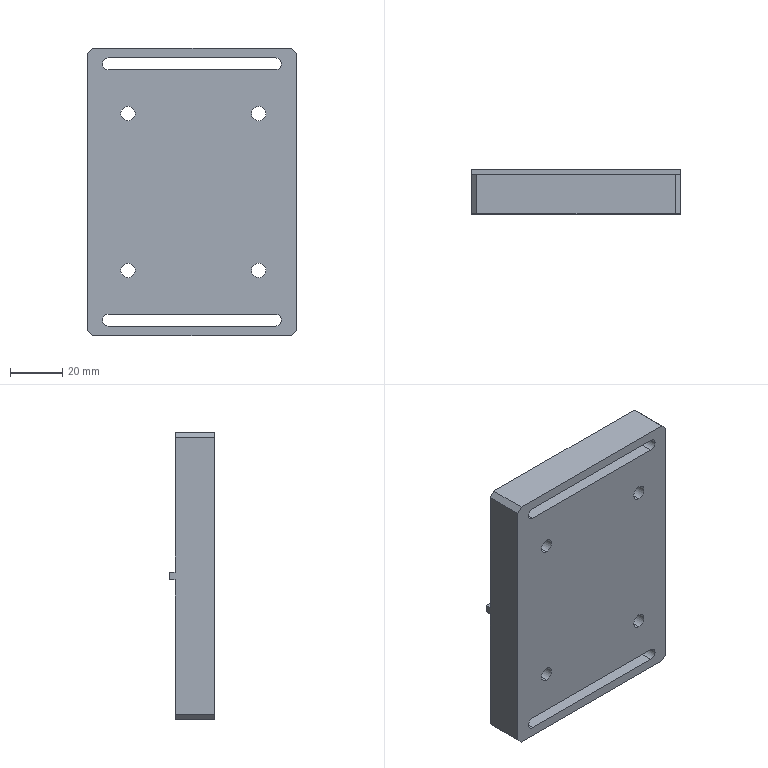Part | STEP file | 11-FG-S01111 | 1 solid | 44 faces | box 80 x 17 x 110 mm | volume 120634 mm3 | cylinder 22 | plane 22 | commonest cylinder face diameters 5.5 x8 10 x8 4.5 x6
STEP:
#1=CARTESIAN_POINT('',(-8.,15.,8.25));
#2=VERTEX_POINT('',#1);
#3=CARTESIAN_POINT('',(-5.75,15.,6.));
#4=VERTEX_POINT('',#3);
#5=CARTESIAN_POINT('',(-8.,15.,6.));
#6=DIRECTION('',(0.,1.,0.));
#7=DIRECTION('',(1.,0.,0.));
#8=AXIS2_PLACEMENT_3D('',#5,#6,#7);
#9=CIRCLE('',#8,2.25);
#10=EDGE_CURVE('',#2,#4,#9,.T.);
#11=ORIENTED_EDGE('',*,*,#10,.T.);
#12=CARTESIAN_POINT('',(-5.75,0.,6.));
#13=VERTEX_POINT('',#12);
#14=CARTESIAN_POINT('',(-5.75,444.,6.));
#15=DIRECTION('',(0.,-1.,0.));
#16=VECTOR('',#15,1000.);
#17=LINE('',#14,#16);
#18=EDGE_CURVE('',#4,#13,#17,.T.);
#19=ORIENTED_EDGE('',*,*,#18,.T.);
#20=CARTESIAN_POINT('',(-8.,0.,8.25));
#21=VERTEX_POINT('',#20);
#22=CARTESIAN_POINT('',(-8.,0.,6.));
#23=DIRECTION('',(0.,1.,0.));
#24=DIRECTION('',(1.,0.,0.));
#25=AXIS2_PLACEMENT_3D('',#22,#23,#24);
#26=CIRCLE('',#25,2.25);
#27=EDGE_CURVE('',#21,#13,#26,.T.);
#28=ORIENTED_EDGE('',*,*,#27,.F.);
#29=CARTESIAN_POINT('',(-8.,444.,8.25));
#30=DIRECTION('',(0.,-1.,0.));
#31=VECTOR('',#30,1000.);
#32=LINE('',#29,#31);
#33=EDGE_CURVE('',#2,#21,#32,.T.);
#34=ORIENTED_EDGE('',*,*,#33,.F.);
#35=EDGE_LOOP('',(#11,#19,#28,#34));
#36=FACE_OUTER_BOUND('',#35,.T.);
#37=CARTESIAN_POINT('',(-8.,444.,6.));
#38=DIRECTION('',(0.,-1.,0.));
#39=DIRECTION('',(1.,0.,0.));
#40=AXIS2_PLACEMENT_3D('',#37,#38,#39);
#41=CYLINDRICAL_SURFACE('',#40,2.25);
#42=ADVANCED_FACE('',(#36),#41,.F.);
#43=CARTESIAN_POINT('',(-5.75,15.,104.));
#44=VERTEX_POINT('',#43);
#45=CARTESIAN_POINT('',(-8.,15.,106.25));
#46=VERTEX_POINT('',#45);
#47=CARTESIAN_POINT('',(-8.,15.,104.));
#48=DIRECTION('',(0.,-1.,0.));
#49=DIRECTION('',(1.,0.,0.));
#50=AXIS2_PLACEMENT_3D('',#47,#48,#49);
#51=CIRCLE('',#50,2.25);
#52=EDGE_CURVE('',#44,#46,#51,.T.);
#53=ORIENTED_EDGE('',*,*,#52,.F.);
#54=CARTESIAN_POINT('',(-5.75,0.,104.));
#55=VERTEX_POINT('',#54);
#56=CARTESIAN_POINT('',(-5.75,444.,104.));
#57=DIRECTION('',(0.,-1.,0.));
#58=VECTOR('',#57,1000.);
#59=LINE('',#56,#58);
#60=EDGE_CURVE('',#44,#55,#59,.T.);
#61=ORIENTED_EDGE('',*,*,#60,.T.);
#62=CARTESIAN_POINT('',(-8.,0.,106.25));
#63=VERTEX_POINT('',#62);
#64=CARTESIAN_POINT('',(-8.,0.,104.));
#65=DIRECTION('',(0.,-1.,0.));
#66=DIRECTION('',(1.,0.,0.));
#67=AXIS2_PLACEMENT_3D('',#64,#65,#66);
#68=CIRCLE('',#67,2.25);
#69=EDGE_CURVE('',#55,#63,#68,.T.);
#70=ORIENTED_EDGE('',*,*,#69,.T.);
#71=CARTESIAN_POINT('',(-8.,444.,106.25));
#72=DIRECTION('',(0.,-1.,0.));
#73=VECTOR('',#72,1000.);
#74=LINE('',#71,#73);
#75=EDGE_CURVE('',#46,#63,#74,.T.);
#76=ORIENTED_EDGE('',*,*,#75,.F.);
#77=EDGE_LOOP('',(#53,#61,#70,#76));
#78=FACE_OUTER_BOUND('',#77,.T.);
#79=CARTESIAN_POINT('',(-8.,444.,104.));
#80=DIRECTION('',(0.,-1.,0.));
#81=DIRECTION('',(1.,0.,0.));
#82=AXIS2_PLACEMENT_3D('',#79,#80,#81);
#83=CYLINDRICAL_SURFACE('',#82,2.25);
#84=ADVANCED_FACE('',(#78),#83,.F.);
#85=CARTESIAN_POINT('',(-14.5,9.6,20.));
#86=VERTEX_POINT('',#85);
#87=CARTESIAN_POINT('',(-14.5,9.6,30.));
#88=VERTEX_POINT('',#87);
#89=CARTESIAN_POINT('',(-14.5,9.6,25.));
#90=DIRECTION('',(0.,1.,0.));
#91=DIRECTION('',(0.,0.,1.));
#92=AXIS2_PLACEMENT_3D('',#89,#90,#91);
#93=CIRCLE('',#92,5.);
#94=EDGE_CURVE('',#86,#88,#93,.T.);
#95=ORIENTED_EDGE('',*,*,#94,.F.);
#96=CARTESIAN_POINT('',(-14.5,15.,20.));
#97=VERTEX_POINT('',#96);
#98=CARTESIAN_POINT('',(-14.5,15.,20.));
#99=DIRECTION('',(0.,1.,0.));
#100=VECTOR('',#99,1000.);
#101=LINE('',#98,#100);
#102=EDGE_CURVE('',#86,#97,#101,.T.);
#103=ORIENTED_EDGE('',*,*,#102,.T.);
#104=CARTESIAN_POINT('',(-14.5,15.,30.));
#105=VERTEX_POINT('',#104);
#106=CARTESIAN_POINT('',(-14.5,15.,25.));
#107=DIRECTION('',(0.,1.,0.));
#108=DIRECTION('',(0.,0.,1.));
#109=AXIS2_PLACEMENT_3D('',#106,#107,#108);
#110=CIRCLE('',#109,5.);
#111=EDGE_CURVE('',#97,#105,#110,.T.);
#112=ORIENTED_EDGE('',*,*,#111,.T.);
#113=CARTESIAN_POINT('',(-14.5,15.,30.));
#114=DIRECTION('',(0.,1.,0.));
#115=VECTOR('',#114,1000.);
#116=LINE('',#113,#115);
#117=EDGE_CURVE('',#88,#105,#116,.T.);
#118=ORIENTED_EDGE('',*,*,#117,.F.);
#119=EDGE_LOOP('',(#95,#103,#112,#118));
#120=FACE_OUTER_BOUND('',#119,.T.);
#121=CARTESIAN_POINT('',(-14.5,15.,25.));
#122=DIRECTION('',(0.,1.,0.));
#123=DIRECTION('',(0.,0.,1.));
#124=AXIS2_PLACEMENT_3D('',#121,#122,#123);
#125=CYLINDRICAL_SURFACE('',#124,5.);
#126=ADVANCED_FACE('',(#120),#125,.F.);
#127=CARTESIAN_POINT('',(-14.5,0.,22.25));
#128=VERTEX_POINT('',#127);
#129=CARTESIAN_POINT('',(-14.5,0.,27.75));
#130=VERTEX_POINT('',#129);
#131=CARTESIAN_POINT('',(-14.5,0.,25.));
#132=DIRECTION('',(0.,1.,0.));
#133=DIRECTION('',(0.,0.,1.));
#134=AXIS2_PLACEMENT_3D('',#131,#132,#133);
#135=CIRCLE('',#134,2.75);
#136=EDGE_CURVE('',#128,#130,#135,.T.);
#137=ORIENTED_EDGE('',*,*,#136,.F.);
#138=CARTESIAN_POINT('',(-14.5,9.6,22.25));
#139=VERTEX_POINT('',#138);
#140=CARTESIAN_POINT('',(-14.5,15.,22.25));
#141=DIRECTION('',(0.,1.,0.));
#142=VECTOR('',#141,1000.);
#143=LINE('',#140,#142);
#144=EDGE_CURVE('',#128,#139,#143,.T.);
#145=ORIENTED_EDGE('',*,*,#144,.T.);
#146=CARTESIAN_POINT('',(-14.5,9.6,27.75));
#147=VERTEX_POINT('',#146);
#148=CARTESIAN_POINT('',(-14.5,9.6,25.));
#149=DIRECTION('',(0.,1.,0.));
#150=DIRECTION('',(0.,0.,1.));
#151=AXIS2_PLACEMENT_3D('',#148,#149,#150);
#152=CIRCLE('',#151,2.75);
#153=EDGE_CURVE('',#139,#147,#152,.T.);
#154=ORIENTED_EDGE('',*,*,#153,.T.);
#155=CARTESIAN_POINT('',(-14.5,15.,27.75));
#156=DIRECTION('',(0.,1.,0.));
#157=VECTOR('',#156,1000.);
#158=LINE('',#155,#157);
#159=EDGE_CURVE('',#130,#147,#158,.T.);
#160=ORIENTED_EDGE('',*,*,#159,.F.);
#161=EDGE_LOOP('',(#137,#145,#154,#160));
#162=FACE_OUTER_BOUND('',#161,.T.);
#163=CARTESIAN_POINT('',(-14.5,15.,25.));
#164=DIRECTION('',(0.,1.,0.));
#165=DIRECTION('',(0.,0.,1.));
#166=AXIS2_PLACEMENT_3D('',#163,#164,#165);
#167=CYLINDRICAL_SURFACE('',#166,2.75);
#168=ADVANCED_FACE('',(#162),#167,.F.);
#169=CARTESIAN_POINT('',(-14.5,9.6,80.));
#170=VERTEX_POINT('',#169);
#171=CARTESIAN_POINT('',(-14.5,9.6,90.));
#172=VERTEX_POINT('',#171);
#173=CARTESIAN_POINT('',(-14.5,9.6,85.));
#174=DIRECTION('',(0.,1.,0.));
#175=DIRECTION('',(0.,0.,1.));
#176=AXIS2_PLACEMENT_3D('',#173,#174,#175);
#177=CIRCLE('',#176,5.);
#178=EDGE_CURVE('',#170,#172,#177,.T.);
#179=ORIENTED_EDGE('',*,*,#178,.F.);
#180=CARTESIAN_POINT('',(-14.5,15.,80.));
#181=VERTEX_POINT('',#180);
#182=CARTESIAN_POINT('',(-14.5,15.,80.));
#183=DIRECTION('',(0.,1.,0.));
#184=VECTOR('',#183,1000.);
#185=LINE('',#182,#184);
#186=EDGE_CURVE('',#170,#181,#185,.T.);
#187=ORIENTED_EDGE('',*,*,#186,.T.);
#188=CARTESIAN_POINT('',(-14.5,15.,90.));
#189=VERTEX_POINT('',#188);
#190=CARTESIAN_POINT('',(-14.5,15.,85.));
#191=DIRECTION('',(0.,1.,0.));
#192=DIRECTION('',(0.,0.,1.));
#193=AXIS2_PLACEMENT_3D('',#190,#191,#192);
#194=CIRCLE('',#193,5.);
#195=EDGE_CURVE('',#181,#189,#194,.T.);
#196=ORIENTED_EDGE('',*,*,#195,.T.);
#197=CARTESIAN_POINT('',(-14.5,15.,90.));
#198=DIRECTION('',(0.,1.,0.));
#199=VECTOR('',#198,1000.);
#200=LINE('',#197,#199);
#201=EDGE_CURVE('',#172,#189,#200,.T.);
#202=ORIENTED_EDGE('',*,*,#201,.F.);
#203=EDGE_LOOP('',(#179,#187,#196,#202));
#204=FACE_OUTER_BOUND('',#203,.T.);
#205=CARTESIAN_POINT('',(-14.5,15.,85.));
#206=DIRECTION('',(0.,1.,0.));
#207=DIRECTION('',(0.,0.,1.));
#208=AXIS2_PLACEMENT_3D('',#205,#206,#207);
#209=CYLINDRICAL_SURFACE('',#208,5.);
#210=ADVANCED_FACE('',(#204),#209,.F.);
#211=CARTESIAN_POINT('',(-14.5,0.,82.25));
#212=VERTEX_POINT('',#211);
#213=CARTESIAN_POINT('',(-14.5,0.,87.75));
#214=VERTEX_POINT('',#213);
#215=CARTESIAN_POINT('',(-14.5,0.,85.));
#216=DIRECTION('',(0.,1.,0.));
#217=DIRECTION('',(0.,0.,1.));
#218=AXIS2_PLACEMENT_3D('',#215,#216,#217);
#219=CIRCLE('',#218,2.75);
#220=EDGE_CURVE('',#212,#214,#219,.T.);
#221=ORIENTED_EDGE('',*,*,#220,.F.);
#222=CARTESIAN_POINT('',(-14.5,9.6,82.25));
#223=VERTEX_POINT('',#222);
#224=CARTESIAN_POINT('',(-14.5,15.,82.25));
#225=DIRECTION('',(0.,1.,0.));
#226=VECTOR('',#225,1000.);
#227=LINE('',#224,#226);
#228=EDGE_CURVE('',#212,#223,#227,.T.);
#229=ORIENTED_EDGE('',*,*,#228,.T.);
#230=CARTESIAN_POINT('',(-14.5,9.6,87.75));
#231=VERTEX_POINT('',#230);
#232=CARTESIAN_POINT('',(-14.5,9.6,85.));
#233=DIRECTION('',(0.,1.,0.));
#234=DIRECTION('',(0.,0.,1.));
#235=AXIS2_PLACEMENT_3D('',#232,#233,#234);
#236=CIRCLE('',#235,2.75);
#237=EDGE_CURVE('',#223,#231,#236,.T.);
#238=ORIENTED_EDGE('',*,*,#237,.T.);
#239=CARTESIAN_POINT('',(-14.5,15.,87.75));
#240=DIRECTION('',(0.,1.,0.));
#241=VECTOR('',#240,1000.);
#242=LINE('',#239,#241);
#243=EDGE_CURVE('',#214,#231,#242,.T.);
#244=ORIENTED_EDGE('',*,*,#243,.F.);
#245=EDGE_LOOP('',(#221,#229,#238,#244));
#246=FACE_OUTER_BOUND('',#245,.T.);
#247=CARTESIAN_POINT('',(-14.5,15.,85.));
#248=DIRECTION('',(0.,1.,0.));
#249=DIRECTION('',(0.,0.,1.));
#250=AXIS2_PLACEMENT_3D('',#247,#248,#249);
#251=CYLINDRICAL_SURFACE('',#250,2.75);
#252=ADVANCED_FACE('',(#246),#251,.F.);
#253=CARTESIAN_POINT('',(-64.5,9.6,20.));
#254=VERTEX_POINT('',#253);
#255=CARTESIAN_POINT('',(-64.5,9.6,30.));
#256=VERTEX_POINT('',#255);
#257=CARTESIAN_POINT('',(-64.5,9.6,25.));
#258=DIRECTION('',(0.,1.,0.));
#259=DIRECTION('',(0.,0.,1.));
#260=AXIS2_PLACEMENT_3D('',#257,#258,#259);
#261=CIRCLE('',#260,5.);
#262=EDGE_CURVE('',#254,#256,#261,.T.);
#263=ORIENTED_EDGE('',*,*,#262,.F.);
#264=CARTESIAN_POINT('',(-64.5,15.,20.));
#265=VERTEX_POINT('',#264);
#266=CARTESIAN_POINT('',(-64.5,15.,20.));
#267=DIRECTION('',(0.,1.,0.));
#268=VECTOR('',#267,1000.);
#269=LINE('',#266,#268);
#270=EDGE_CURVE('',#254,#265,#269,.T.);
#271=ORIENTED_EDGE('',*,*,#270,.T.);
#272=CARTESIAN_POINT('',(-64.5,15.,30.));
#273=VERTEX_POINT('',#272);
#274=CARTESIAN_POINT('',(-64.5,15.,25.));
#275=DIRECTION('',(0.,1.,0.));
#276=DIRECTION('',(0.,0.,1.));
#277=AXIS2_PLACEMENT_3D('',#274,#275,#276);
#278=CIRCLE('',#277,5.);
#279=EDGE_CURVE('',#265,#273,#278,.T.);
#280=ORIENTED_EDGE('',*,*,#279,.T.);
#281=CARTESIAN_POINT('',(-64.5,15.,30.));
#282=DIRECTION('',(0.,1.,0.));
#283=VECTOR('',#282,1000.);
#284=LINE('',#281,#283);
#285=EDGE_CURVE('',#256,#273,#284,.T.);
#286=ORIENTED_EDGE('',*,*,#285,.F.);
#287=EDGE_LOOP('',(#263,#271,#280,#286));
#288=FACE_OUTER_BOUND('',#287,.T.);
#289=CARTESIAN_POINT('',(-64.5,15.,25.));
#290=DIRECTION('',(0.,1.,0.));
#291=DIRECTION('',(0.,0.,1.));
#292=AXIS2_PLACEMENT_3D('',#289,#290,#291);
#293=CYLINDRICAL_SURFACE('',#292,5.);
#294=ADVANCED_FACE('',(#288),#293,.F.);
#295=CARTESIAN_POINT('',(-64.5,0.,22.25));
#296=VERTEX_POINT('',#295);
#297=CARTESIAN_POINT('',(-64.5,0.,27.75));
#298=VERTEX_POINT('',#297);
#299=CARTESIAN_POINT('',(-64.5,0.,25.));
#300=DIRECTION('',(0.,1.,0.));
#301=DIRECTION('',(0.,0.,1.));
#302=AXIS2_PLACEMENT_3D('',#299,#300,#301);
#303=CIRCLE('',#302,2.75);
#304=EDGE_CURVE('',#296,#298,#303,.T.);
#305=ORIENTED_EDGE('',*,*,#304,.F.);
#306=CARTESIAN_POINT('',(-64.5,9.6,22.25));
#307=VERTEX_POINT('',#306);
#308=CARTESIAN_POINT('',(-64.5,15.,22.25));
#309=DIRECTION('',(0.,1.,0.));
#310=VECTOR('',#309,1000.);
#311=LINE('',#308,#310);
#312=EDGE_CURVE('',#296,#307,#311,.T.);
#313=ORIENTED_EDGE('',*,*,#312,.T.);
#314=CARTESIAN_POINT('',(-64.5,9.6,27.75));
#315=VERTEX_POINT('',#314);
#316=CARTESIAN_POINT('',(-64.5,9.6,25.));
#317=DIRECTION('',(0.,1.,0.));
#318=DIRECTION('',(0.,0.,1.));
#319=AXIS2_PLACEMENT_3D('',#316,#317,#318);
#320=CIRCLE('',#319,2.75);
#321=EDGE_CURVE('',#307,#315,#320,.T.);
#322=ORIENTED_EDGE('',*,*,#321,.T.);
#323=CARTESIAN_POINT('',(-64.5,15.,27.75));
#324=DIRECTION('',(0.,1.,0.));
#325=VECTOR('',#324,1000.);
#326=LINE('',#323,#325);
#327=EDGE_CURVE('',#298,#315,#326,.T.);
#328=ORIENTED_EDGE('',*,*,#327,.F.);
#329=EDGE_LOOP('',(#305,#313,#322,#328));
#330=FACE_OUTER_BOUND('',#329,.T.);
#331=CARTESIAN_POINT('',(-64.5,15.,25.));
#332=DIRECTION('',(0.,1.,0.));
#333=DIRECTION('',(0.,0.,1.));
#334=AXIS2_PLACEMENT_3D('',#331,#332,#333);
#335=CYLINDRICAL_SURFACE('',#334,2.75);
#336=ADVANCED_FACE('',(#330),#335,.F.);
#337=CARTESIAN_POINT('',(-64.5,9.6,80.));
#338=VERTEX_POINT('',#337);
#339=CARTESIAN_POINT('',(-64.5,9.6,90.));
#340=VERTEX_POINT('',#339);
#341=CARTESIAN_POINT('',(-64.5,9.6,85.));
#342=DIRECTION('',(0.,1.,0.));
#343=DIRECTION('',(0.,0.,1.));
#344=AXIS2_PLACEMENT_3D('',#341,#342,#343);
#345=CIRCLE('',#344,5.);
#346=EDGE_CURVE('',#338,#340,#345,.T.);
#347=ORIENTED_EDGE('',*,*,#346,.F.);
#348=CARTESIAN_POINT('',(-64.5,15.,80.));
#349=VERTEX_POINT('',#348);
#350=CARTESIAN_POINT('',(-64.5,15.,80.));
#351=DIRECTION('',(0.,1.,0.));
#352=VECTOR('',#351,1000.);
#353=LINE('',#350,#352);
#354=EDGE_CURVE('',#338,#349,#353,.T.);
#355=ORIENTED_EDGE('',*,*,#354,.T.);
#356=CARTESIAN_POINT('',(-64.5,15.,90.));
#357=VERTEX_POINT('',#356);
#358=CARTESIAN_POINT('',(-64.5,15.,85.));
#359=DIRECTION('',(0.,1.,0.));
#360=DIRECTION('',(0.,0.,1.));
#361=AXIS2_PLACEMENT_3D('',#358,#359,#360);
#362=CIRCLE('',#361,5.);
#363=EDGE_CURVE('',#349,#357,#362,.T.);
#364=ORIENTED_EDGE('',*,*,#363,.T.);
#365=CARTESIAN_POINT('',(-64.5,15.,90.));
#366=DIRECTION('',(0.,1.,0.));
#367=VECTOR('',#366,1000.);
#368=LINE('',#365,#367);
#369=EDGE_CURVE('',#340,#357,#368,.T.);
#370=ORIENTED_EDGE('',*,*,#369,.F.);
#371=EDGE_LOOP('',(#347,#355,#364,#370));
#372=FACE_OUTER_BOUND('',#371,.T.);
#373=CARTESIAN_POINT('',(-64.5,15.,85.));
#374=DIRECTION('',(0.,1.,0.));
#375=DIRECTION('',(0.,0.,1.));
#376=AXIS2_PLACEMENT_3D('',#373,#374,#375);
#377=CYLINDRICAL_SURFACE('',#376,5.);
#378=ADVANCED_FACE('',(#372),#377,.F.);
#379=CARTESIAN_POINT('',(-64.5,0.,82.25));
#380=VERTEX_POINT('',#379);
#381=CARTESIAN_POINT('',(-64.5,0.,87.75));
#382=VERTEX_POINT('',#381);
#383=CARTESIAN_POINT('',(-64.5,0.,85.));
#384=DIRECTION('',(0.,1.,0.));
#385=DIRECTION('',(0.,0.,1.));
#386=AXIS2_PLACEMENT_3D('',#383,#384,#385);
#387=CIRCLE('',#386,2.75);
#388=EDGE_CURVE('',#380,#382,#387,.T.);
#389=ORIENTED_EDGE('',*,*,#388,.F.);
#390=CARTESIAN_POINT('',(-64.5,9.6,82.25));
#391=VERTEX_POINT('',#390);
#392=CARTESIAN_POINT('',(-64.5,15.,82.25));
#393=DIRECTION('',(0.,1.,0.));
#394=VECTOR('',#393,1000.);
#395=LINE('',#392,#394);
#396=EDGE_CURVE('',#380,#391,#395,.T.);
#397=ORIENTED_EDGE('',*,*,#396,.T.);
#398=CARTESIAN_POINT('',(-64.5,9.6,87.75));
#399=VERTEX_POINT('',#398);
#400=CARTESIAN_POINT('',(-64.5,9.6,85.));
#401=DIRECTION('',(0.,1.,0.));
#402=DIRECTION('',(0.,0.,1.));
#403=AXIS2_PLACEMENT_3D('',#400,#401,#402);
#404=CIRCLE('',#403,2.75);
#405=EDGE_CURVE('',#391,#399,#404,.T.);
#406=ORIENTED_EDGE('',*,*,#405,.T.);
#407=CARTESIAN_POINT('',(-64.5,15.,87.75));
#408=DIRECTION('',(0.,1.,0.));
#409=VECTOR('',#408,1000.);
#410=LINE('',#407,#409);
#411=EDGE_CURVE('',#382,#399,#410,.T.);
#412=ORIENTED_EDGE('',*,*,#411,.F.);
#413=EDGE_LOOP('',(#389,#397,#406,#412));
#414=FACE_OUTER_BOUND('',#413,.T.);
#415=CARTESIAN_POINT('',(-64.5,15.,85.));
#416=DIRECTION('',(0.,1.,0.));
#417=DIRECTION('',(0.,0.,1.));
#418=AXIS2_PLACEMENT_3D('',#415,#416,#417);
#419=CYLINDRICAL_SURFACE('',#418,2.75);
#420=ADVANCED_FACE('',(#414),#419,.F.);
#421=CARTESIAN_POINT('',(-80.,15.,53.5));
#422=VERTEX_POINT('',#421);
#423=CARTESIAN_POINT('',(-80.,15.,2.));
#424=VERTEX_POINT('',#423);
#425=CARTESIAN_POINT('',(-80.,15.,110.));
#426=DIRECTION('',(0.,0.,-1.));
#427=VECTOR('',#426,1000.);
#428=LINE('',#425,#427);
#429=EDGE_CURVE('',#422,#424,#428,.T.);
#430=ORIENTED_EDGE('',*,*,#429,.F.);
#431=CARTESIAN_POINT('',(0.,15.,53.5));
#432=VERTEX_POINT('',#431);
#433=CARTESIAN_POINT('',(-83.606,15.,53.5));
#434=DIRECTION('',(1.,0.,0.));
#435=VECTOR('',#434,1000.);
#436=LINE('',#433,#435);
#437=EDGE_CURVE('',#422,#432,#436,.T.);
#438=ORIENTED_EDGE('',*,*,#437,.T.);
#439=CARTESIAN_POINT('',(0.,15.,2.));
#440=VERTEX_POINT('',#439);
#441=CARTESIAN_POINT('',(0.,15.,110.));
#442=DIRECTION('',(0.,0.,-1.));
#443=VECTOR('',#442,1000.);
#444=LINE('',#441,#443);
#445=EDGE_CURVE('',#432,#440,#444,.T.);
#446=ORIENTED_EDGE('',*,*,#445,.T.);
#447=CARTESIAN_POINT('',(-2.,15.,0.));
#448=VERTEX_POINT('',#447);
#449=CARTESIAN_POINT('',(0.,15.,2.));
#450=DIRECTION('',(-0.7071,0.,-0.7071));
#451=VECTOR('',#450,1000.);
#452=LINE('',#449,#451);
#453=EDGE_CURVE('',#440,#448,#452,.T.);
#454=ORIENTED_EDGE('',*,*,#453,.T.);
#455=CARTESIAN_POINT('',(-78.,15.,0.));
#456=VERTEX_POINT('',#455);
#457=CARTESIAN_POINT('',(0.,15.,0.));
#458=DIRECTION('',(-1.,0.,0.));
#459=VECTOR('',#458,1000.);
#460=LINE('',#457,#459);
#461=EDGE_CURVE('',#448,#456,#460,.T.);
#462=ORIENTED_EDGE('',*,*,#461,.T.);
#463=CARTESIAN_POINT('',(-80.,15.,2.));
#464=DIRECTION('',(-0.7071,0.,0.7071));
#465=VECTOR('',#464,1000.);
#466=LINE('',#463,#465);
#467=EDGE_CURVE('',#456,#424,#466,.T.);
#468=ORIENTED_EDGE('',*,*,#467,.T.);
#469=EDGE_LOOP('',(#430,#438,#446,#454,#462,#468));
#470=FACE_OUTER_BOUND('',#469,.T.);
#471=CARTESIAN_POINT('',(-64.5,15.,25.));
#472=DIRECTION('',(0.,1.,0.));
#473=DIRECTION('',(0.,0.,1.));
#474=AXIS2_PLACEMENT_3D('',#471,#472,#473);
#475=CIRCLE('',#474,5.);
#476=EDGE_CURVE('',#273,#265,#475,.T.);
#477=ORIENTED_EDGE('',*,*,#476,.F.);
#478=ORIENTED_EDGE('',*,*,#279,.F.);
#479=EDGE_LOOP('',(#477,#478));
#480=FACE_BOUND('',#479,.T.);
#481=CARTESIAN_POINT('',(-14.5,15.,25.));
#482=DIRECTION('',(0.,1.,0.));
#483=DIRECTION('',(0.,0.,1.));
#484=AXIS2_PLACEMENT_3D('',#481,#482,#483);
#485=CIRCLE('',#484,5.);
#486=EDGE_CURVE('',#105,#97,#485,.T.);
#487=ORIENTED_EDGE('',*,*,#486,.F.);
#488=ORIENTED_EDGE('',*,*,#111,.F.);
#489=EDGE_LOOP('',(#487,#488));
#490=FACE_BOUND('',#489,.T.);
#491=ORIENTED_EDGE('',*,*,#10,.F.);
#492=CARTESIAN_POINT('',(-72.,15.,8.25));
#493=VERTEX_POINT('',#492);
#494=CARTESIAN_POINT('',(0.,15.,8.25));
#495=DIRECTION('',(1.,0.,0.));
#496=VECTOR('',#495,1000.);
#497=LINE('',#494,#496);
#498=EDGE_CURVE('',#493,#2,#497,.T.);
#499=ORIENTED_EDGE('',*,*,#498,.F.);
#500=CARTESIAN_POINT('',(-72.,15.,3.75));
#501=VERTEX_POINT('',#500);
#502=CARTESIAN_POINT('',(-72.,15.,6.));
#503=DIRECTION('',(0.,1.,0.));
#504=DIRECTION('',(1.,0.,0.));
#505=AXIS2_PLACEMENT_3D('',#502,#503,#504);
#506=CIRCLE('',#505,2.25);
#507=EDGE_CURVE('',#501,#493,#506,.T.);
#508=ORIENTED_EDGE('',*,*,#507,.F.);
#509=CARTESIAN_POINT('',(-8.,15.,3.75));
#510=VERTEX_POINT('',#509);
#511=CARTESIAN_POINT('',(0.,15.,3.75));
#512=DIRECTION('',(-1.,0.,0.));
#513=VECTOR('',#512,1000.);
#514=LINE('',#511,#513);
#515=EDGE_CURVE('',#510,#501,#514,.T.);
#516=ORIENTED_EDGE('',*,*,#515,.F.);
#517=CARTESIAN_POINT('',(-8.,15.,6.));
#518=DIRECTION('',(0.,1.,0.));
#519=DIRECTION('',(1.,0.,0.));
#520=AXIS2_PLACEMENT_3D('',#517,#518,#519);
#521=CIRCLE('',#520,2.25);
#522=EDGE_CURVE('',#4,#510,#521,.T.);
#523=ORIENTED_EDGE('',*,*,#522,.F.);
#524=EDGE_LOOP('',(#491,#499,#508,#516,#523));
#525=FACE_BOUND('',#524,.T.);
#526=CARTESIAN_POINT('',(0.,15.,110.));
#527=DIRECTION('',(0.,-1.,0.));
#528=DIRECTION('',(1.,0.,0.));
#529=AXIS2_PLACEMENT_3D('',#526,#527,#528);
#530=PLANE('',#529);
#531=ADVANCED_FACE('',(#470,#480,#490,#525),#530,.F.);
#532=CARTESIAN_POINT('',(-78.,0.,110.));
#533=VERTEX_POINT('',#532);
#534=CARTESIAN_POINT('',(-2.,0.,110.));
#535=VERTEX_POINT('',#534);
#536=CARTESIAN_POINT('',(0.,0.,110.));
#537=DIRECTION('',(1.,0.,0.));
#538=VECTOR('',#537,1000.);
#539=LINE('',#536,#538);
#540=EDGE_CURVE('',#533,#535,#539,.T.);
#541=ORIENTED_EDGE('',*,*,#540,.F.);
#542=CARTESIAN_POINT('',(-80.,0.,108.));
#543=VERTEX_POINT('',#542);
#544=CARTESIAN_POINT('',(-78.,0.,110.));
#545=DIRECTION('',(-0.7071,0.,-0.7071));
#546=VECTOR('',#545,1000.);
#547=LINE('',#544,#546);
#548=EDGE_CURVE('',#533,#543,#547,.T.);
#549=ORIENTED_EDGE('',*,*,#548,.T.);
#550=CARTESIAN_POINT('',(-80.,0.,2.));
#551=VERTEX_POINT('',#550);
#552=CARTESIAN_POINT('',(-80.,0.,110.));
#553=DIRECTION('',(0.,0.,-1.));
#554=VECTOR('',#553,1000.);
#555=LINE('',#552,#554);
#556=EDGE_CURVE('',#543,#551,#555,.T.);
#557=ORIENTED_EDGE('',*,*,#556,.T.);
#558=CARTESIAN_POINT('',(-78.,0.,0.));
#559=VERTEX_POINT('',#558);
#560=CARTESIAN_POINT('',(-80.,0.,2.));
#561=DIRECTION('',(0.7071,0.,-0.7071));
#562=VECTOR('',#561,1000.);
#563=LINE('',#560,#562);
#564=EDGE_CURVE('',#551,#559,#563,.T.);
#565=ORIENTED_EDGE('',*,*,#564,.T.);
#566=CARTESIAN_POINT('',(-2.,0.,0.));
#567=VERTEX_POINT('',#566);
#568=CARTESIAN_POINT('',(0.,0.,0.));
#569=DIRECTION('',(1.,0.,0.));
#570=VECTOR('',#569,1000.);
#571=LINE('',#568,#570);
#572=EDGE_CURVE('',#559,#567,#571,.T.);
#573=ORIENTED_EDGE('',*,*,#572,.T.);
#574=CARTESIAN_POINT('',(0.,0.,2.));
#575=VERTEX_POINT('',#574);
#576=CARTESIAN_POINT('',(0.,0.,2.));
#577=DIRECTION('',(0.7071,0.,0.7071));
#578=VECTOR('',#577,1000.);
#579=LINE('',#576,#578);
#580=EDGE_CURVE('',#567,#575,#579,.T.);
#581=ORIENTED_EDGE('',*,*,#580,.T.);
#582=CARTESIAN_POINT('',(0.,0.,108.));
#583=VERTEX_POINT('',#582);
#584=CARTESIAN_POINT('',(0.,0.,110.));
#585=DIRECTION('',(0.,0.,-1.));
#586=VECTOR('',#585,1000.);
#587=LINE('',#584,#586);
#588=EDGE_CURVE('',#583,#575,#587,.T.);
#589=ORIENTED_EDGE('',*,*,#588,.F.);
#590=CARTESIAN_POINT('',(-2.,0.,110.));
#591=DIRECTION('',(-0.7071,0.,0.7071));
#592=VECTOR('',#591,1000.);
#593=LINE('',#590,#592);
#594=EDGE_CURVE('',#583,#535,#593,.T.);
#595=ORIENTED_EDGE('',*,*,#594,.T.);
#596=EDGE_LOOP('',(#541,#549,#557,#565,#573,#581,#589,#595));
#597=FACE_OUTER_BOUND('',#596,.T.);
#598=CARTESIAN_POINT('',(-64.5,0.,85.));
#599=DIRECTION('',(0.,1.,0.));
#600=DIRECTION('',(0.,0.,1.));
#601=AXIS2_PLACEMENT_3D('',#598,#599,#600);
#602=CIRCLE('',#601,2.75);
#603=EDGE_CURVE('',#382,#380,#602,.T.);
#604=ORIENTED_EDGE('',*,*,#603,.T.);
#605=ORIENTED_EDGE('',*,*,#388,.T.);
#606=EDGE_LOOP('',(#604,#605));
#607=FACE_BOUND('',#606,.T.);
#608=CARTESIAN_POINT('',(-64.5,0.,25.));
#609=DIRECTION('',(0.,1.,0.));
#610=DIRECTION('',(0.,0.,1.));
#611=AXIS2_PLACEMENT_3D('',#608,#609,#610);
#612=CIRCLE('',#611,2.75);
#613=EDGE_CURVE('',#298,#296,#612,.T.);
#614=ORIENTED_EDGE('',*,*,#613,.T.);
#615=ORIENTED_EDGE('',*,*,#304,.T.);
#616=EDGE_LOOP('',(#614,#615));
#617=FACE_BOUND('',#616,.T.);
#618=CARTESIAN_POINT('',(-14.5,0.,85.));
#619=DIRECTION('',(0.,1.,0.));
#620=DIRECTION('',(0.,0.,1.));
#621=AXIS2_PLACEMENT_3D('',#618,#619,#620);
#622=CIRCLE('',#621,2.75);
#623=EDGE_CURVE('',#214,#212,#622,.T.);
#624=ORIENTED_EDGE('',*,*,#623,.T.);
#625=ORIENTED_EDGE('',*,*,#220,.T.);
#626=EDGE_LOOP('',(#624,#625));
#627=FACE_BOUND('',#626,.T.);
#628=CARTESIAN_POINT('',(-14.5,0.,25.));
#629=DIRECTION('',(0.,1.,0.));
#630=DIRECTION('',(0.,0.,1.));
#631=AXIS2_PLACEMENT_3D('',#628,#629,#630);
#632=CIRCLE('',#631,2.75);
#633=EDGE_CURVE('',#130,#128,#632,.T.);
#634=ORIENTED_EDGE('',*,*,#633,.T.);
#635=ORIENTED_EDGE('',*,*,#136,.T.);
#636=EDGE_LOOP('',(#634,#635));
#637=FACE_BOUND('',#636,.T.);
#638=CARTESIAN_POINT('',(-72.,0.,106.25));
#639=VERTEX_POINT('',#638);
#640=CARTESIAN_POINT('',(-8.,0.,106.25));
#641=DIRECTION('',(-1.,0.,0.));
#642=VECTOR('',#641,1000.);
#643=LINE('',#640,#642);
#644=EDGE_CURVE('',#63,#639,#643,.T.);
#645=ORIENTED_EDGE('',*,*,#644,.F.);
#646=ORIENTED_EDGE('',*,*,#69,.F.);
#647=CARTESIAN_POINT('',(-8.,0.,101.75));
#648=VERTEX_POINT('',#647);
#649=CARTESIAN_POINT('',(-8.,0.,104.));
#650=DIRECTION('',(0.,-1.,0.));
#651=DIRECTION('',(1.,0.,0.));
#652=AXIS2_PLACEMENT_3D('',#649,#650,#651);
#653=CIRCLE('',#652,2.25);
#654=EDGE_CURVE('',#648,#55,#653,.T.);
#655=ORIENTED_EDGE('',*,*,#654,.F.);
#656=CARTESIAN_POINT('',(-72.,0.,101.75));
#657=VERTEX_POINT('',#656);
#658=CARTESIAN_POINT('',(-8.,0.,101.75));
#659=DIRECTION('',(1.,0.,0.));
#660=VECTOR('',#659,1000.);
#661=LINE('',#658,#660);
#662=EDGE_CURVE('',#657,#648,#661,.T.);
#663=ORIENTED_EDGE('',*,*,#662,.F.);
#664=CARTESIAN_POINT('',(-72.,0.,104.));
#665=DIRECTION('',(0.,-1.,0.));
#666=DIRECTION('',(1.,0.,0.));
#667=AXIS2_PLACEMENT_3D('',#664,#665,#666);
#668=CIRCLE('',#667,2.25);
#669=EDGE_CURVE('',#639,#657,#668,.T.);
#670=ORIENTED_EDGE('',*,*,#669,.F.);
#671=EDGE_LOOP('',(#645,#646,#655,#663,#670));
#672=FACE_BOUND('',#671,.T.);
#673=ORIENTED_EDGE('',*,*,#27,.T.);
#674=CARTESIAN_POINT('',(-8.,0.,3.75));
#675=VERTEX_POINT('',#674);
#676=CARTESIAN_POINT('',(-8.,0.,6.));
#677=DIRECTION('',(0.,1.,0.));
#678=DIRECTION('',(1.,0.,0.));
#679=AXIS2_PLACEMENT_3D('',#676,#677,#678);
#680=CIRCLE('',#679,2.25);
#681=EDGE_CURVE('',#13,#675,#680,.T.);
#682=ORIENTED_EDGE('',*,*,#681,.T.);
#683=CARTESIAN_POINT('',(-72.,0.,3.75));
#684=VERTEX_POINT('',#683);
#685=CARTESIAN_POINT('',(-8.,0.,3.75));
#686=DIRECTION('',(-1.,0.,0.));
#687=VECTOR('',#686,1000.);
#688=LINE('',#685,#687);
#689=EDGE_CURVE('',#675,#684,#688,.T.);
#690=ORIENTED_EDGE('',*,*,#689,.T.);
#691=CARTESIAN_POINT('',(-72.,0.,8.25));
#692=VERTEX_POINT('',#691);
#693=CARTESIAN_POINT('',(-72.,0.,6.));
#694=DIRECTION('',(0.,1.,0.));
#695=DIRECTION('',(1.,0.,0.));
#696=AXIS2_PLACEMENT_3D('',#693,#694,#695);
#697=CIRCLE('',#696,2.25);
#698=EDGE_CURVE('',#684,#692,#697,.T.);
#699=ORIENTED_EDGE('',*,*,#698,.T.);
#700=CARTESIAN_POINT('',(-8.,0.,8.25));
#701=DIRECTION('',(1.,0.,0.));
#702=VECTOR('',#701,1000.);
#703=LINE('',#700,#702);
#704=EDGE_CURVE('',#692,#21,#703,.T.);
#705=ORIENTED_EDGE('',*,*,#704,.T.);
#706=EDGE_LOOP('',(#673,#682,#690,#699,#705));
#707=FACE_BOUND('',#706,.T.);
#708=CARTESIAN_POINT('',(0.,0.,110.));
#709=DIRECTION('',(0.,1.,0.));
#710=DIRECTION('',(-1.,0.,0.));
#711=AXIS2_PLACEMENT_3D('',#708,#709,#710);
#712=PLANE('',#711);
#713=ADVANCED_FACE('',(#597,#607,#617,#627,#637,#672,#707),#712,.F.);
#714=CARTESIAN_POINT('',(-72.,15.,101.75));
#715=VERTEX_POINT('',#714);
#716=CARTESIAN_POINT('',(-8.,15.,101.75));
#717=VERTEX_POINT('',#716);
#718=CARTESIAN_POINT('',(0.,15.,101.75));
#719=DIRECTION('',(1.,0.,0.));
#720=VECTOR('',#719,1000.);
#721=LINE('',#718,#720);
#722=EDGE_CURVE('',#715,#717,#721,.T.);
#723=ORIENTED_EDGE('',*,*,#722,.T.);
#724=CARTESIAN_POINT('',(-8.,15.,104.));
#725=DIRECTION('',(0.,-1.,0.));
#726=DIRECTION('',(1.,0.,0.));
#727=AXIS2_PLACEMENT_3D('',#724,#725,#726);
#728=CIRCLE('',#727,2.25);
#729=EDGE_CURVE('',#717,#44,#728,.T.);
#730=ORIENTED_EDGE('',*,*,#729,.T.);
#731=ORIENTED_EDGE('',*,*,#52,.T.);
#732=CARTESIAN_POINT('',(-72.,15.,106.25));
#733=VERTEX_POINT('',#732);
#734=CARTESIAN_POINT('',(0.,15.,106.25));
#735=DIRECTION('',(-1.,0.,0.));
#736=VECTOR('',#735,1000.);
#737=LINE('',#734,#736);
#738=EDGE_CURVE('',#46,#733,#737,.T.);
#739=ORIENTED_EDGE('',*,*,#738,.T.);
#740=CARTESIAN_POINT('',(-72.,15.,104.));
#741=DIRECTION('',(0.,-1.,0.));
#742=DIRECTION('',(1.,0.,0.));
#743=AXIS2_PLACEMENT_3D('',#740,#741,#742);
#744=CIRCLE('',#743,2.25);
#745=EDGE_CURVE('',#733,#715,#744,.T.);
#746=ORIENTED_EDGE('',*,*,#745,.T.);
#747=EDGE_LOOP('',(#723,#730,#731,#739,#746));
#748=FACE_BOUND('',#747,.T.);
#749=CARTESIAN_POINT('',(-64.5,15.,85.));
#750=DIRECTION('',(0.,1.,0.));
#751=DIRECTION('',(0.,0.,1.));
#752=AXIS2_PLACEMENT_3D('',#749,#750,#751);
#753=CIRCLE('',#752,5.);
#754=EDGE_CURVE('',#357,#349,#753,.T.);
#755=ORIENTED_EDGE('',*,*,#754,.F.);
#756=ORIENTED_EDGE('',*,*,#363,.F.);
#757=EDGE_LOOP('',(#755,#756));
#758=FACE_BOUND('',#757,.T.);
#759=CARTESIAN_POINT('',(-14.5,15.,85.));
#760=DIRECTION('',(0.,1.,0.));
#761=DIRECTION('',(0.,0.,1.));
#762=AXIS2_PLACEMENT_3D('',#759,#760,#761);
#763=CIRCLE('',#762,5.);
#764=EDGE_CURVE('',#189,#181,#763,.T.);
#765=ORIENTED_EDGE('',*,*,#764,.F.);
#766=ORIENTED_EDGE('',*,*,#195,.F.);
#767=EDGE_LOOP('',(#765,#766));
#768=FACE_BOUND('',#767,.T.);
#769=CARTESIAN_POINT('',(-80.,15.,56.5));
#770=VERTEX_POINT('',#769);
#771=CARTESIAN_POINT('',(0.,15.,56.5));
#772=VERTEX_POINT('',#771);
#773=CARTESIAN_POINT('',(-83.606,15.,56.5));
#774=DIRECTION('',(1.,0.,0.));
#775=VECTOR('',#774,1000.);
#776=LINE('',#773,#775);
#777=EDGE_CURVE('',#770,#772,#776,.T.);
#778=ORIENTED_EDGE('',*,*,#777,.F.);
#779=CARTESIAN_POINT('',(-80.,15.,108.));
#780=VERTEX_POINT('',#779);
#781=CARTESIAN_POINT('',(-80.,15.,110.));
#782=DIRECTION('',(0.,0.,-1.));
#783=VECTOR('',#782,1000.);
#784=LINE('',#781,#783);
#785=EDGE_CURVE('',#780,#770,#784,.T.);
#786=ORIENTED_EDGE('',*,*,#785,.F.);
#787=CARTESIAN_POINT('',(-78.,15.,110.));
#788=VERTEX_POINT('',#787);
#789=CARTESIAN_POINT('',(-78.,15.,110.));
#790=DIRECTION('',(0.7071,0.,0.7071));
#791=VECTOR('',#790,1000.);
#792=LINE('',#789,#791);
#793=EDGE_CURVE('',#780,#788,#792,.T.);
#794=ORIENTED_EDGE('',*,*,#793,.T.);
#795=CARTESIAN_POINT('',(-2.,15.,110.));
#796=VERTEX_POINT('',#795);
#797=CARTESIAN_POINT('',(0.,15.,110.));
#798=DIRECTION('',(-1.,0.,0.));
#799=VECTOR('',#798,1000.);
#800=LINE('',#797,#799);
#801=EDGE_CURVE('',#796,#788,#800,.T.);
#802=ORIENTED_EDGE('',*,*,#801,.F.);
#803=CARTESIAN_POINT('',(0.,15.,108.));
#804=VERTEX_POINT('',#803);
#805=CARTESIAN_POINT('',(-2.,15.,110.));
#806=DIRECTION('',(0.7071,0.,-0.7071));
#807=VECTOR('',#806,1000.);
#808=LINE('',#805,#807);
#809=EDGE_CURVE('',#796,#804,#808,.T.);
#810=ORIENTED_EDGE('',*,*,#809,.T.);
#811=CARTESIAN_POINT('',(0.,15.,110.));
#812=DIRECTION('',(0.,0.,-1.));
#813=VECTOR('',#812,1000.);
#814=LINE('',#811,#813);
#815=EDGE_CURVE('',#804,#772,#814,.T.);
#816=ORIENTED_EDGE('',*,*,#815,.T.);
#817=EDGE_LOOP('',(#778,#786,#794,#802,#810,#816));
#818=FACE_OUTER_BOUND('',#817,.T.);
#819=CARTESIAN_POINT('',(0.,15.,110.));
#820=DIRECTION('',(0.,-1.,0.));
#821=DIRECTION('',(1.,0.,0.));
#822=AXIS2_PLACEMENT_3D('',#819,#820,#821);
#823=PLANE('',#822);
#824=ADVANCED_FACE('',(#748,#758,#768,#818),#823,.F.);
#825=ORIENTED_EDGE('',*,*,#815,.F.);
#826=CARTESIAN_POINT('',(0.,0.,108.));
#827=DIRECTION('',(0.,-1.,0.));
#828=VECTOR('',#827,1000.);
#829=LINE('',#826,#828);
#830=EDGE_CURVE('',#804,#583,#829,.T.);
#831=ORIENTED_EDGE('',*,*,#830,.T.);
#832=ORIENTED_EDGE('',*,*,#588,.T.);
#833=CARTESIAN_POINT('',(0.,0.,2.));
#834=DIRECTION('',(0.,1.,0.));
#835=VECTOR('',#834,1000.);
#836=LINE('',#833,#835);
#837=EDGE_CURVE('',#575,#440,#836,.T.);
#838=ORIENTED_EDGE('',*,*,#837,.T.);
#839=ORIENTED_EDGE('',*,*,#445,.F.);
#840=CARTESIAN_POINT('',(0.,17.,53.5));
#841=VERTEX_POINT('',#840);
#842=CARTESIAN_POINT('',(0.,15.,53.5));
#843=DIRECTION('',(0.,1.,0.));
#844=VECTOR('',#843,1000.);
#845=LINE('',#842,#844);
#846=EDGE_CURVE('',#432,#841,#845,.T.);
#847=ORIENTED_EDGE('',*,*,#846,.T.);
#848=CARTESIAN_POINT('',(0.,17.,56.5));
#849=VERTEX_POINT('',#848);
#850=CARTESIAN_POINT('',(0.,17.,53.5));
#851=DIRECTION('',(0.,0.,1.));
#852=VECTOR('',#851,1000.);
#853=LINE('',#850,#852);
#854=EDGE_CURVE('',#841,#849,#853,.T.);
#855=ORIENTED_EDGE('',*,*,#854,.T.);
#856=CARTESIAN_POINT('',(0.,15.,56.5));
#857=DIRECTION('',(0.,-1.,0.));
#858=VECTOR('',#857,1000.);
#859=LINE('',#856,#858);
#860=EDGE_CURVE('',#849,#772,#859,.T.);
#861=ORIENTED_EDGE('',*,*,#860,.T.);
#862=EDGE_LOOP('',(#825,#831,#832,#838,#839,#847,#855,#861));
#863=FACE_OUTER_BOUND('',#862,.T.);
#864=CARTESIAN_POINT('',(0.,0.,110.));
#865=DIRECTION('',(-1.,0.,0.));
#866=DIRECTION('',(0.,0.,1.));
#867=AXIS2_PLACEMENT_3D('',#864,#865,#866);
#868=PLANE('',#867);
#869=ADVANCED_FACE('',(#863),#868,.F.);
#870=ORIENTED_EDGE('',*,*,#556,.F.);
#871=CARTESIAN_POINT('',(-80.,15.,108.));
#872=DIRECTION('',(0.,1.,0.));
#873=VECTOR('',#872,1000.);
#874=LINE('',#871,#873);
#875=EDGE_CURVE('',#543,#780,#874,.T.);
#876=ORIENTED_EDGE('',*,*,#875,.T.);
#877=ORIENTED_EDGE('',*,*,#785,.T.);
#878=CARTESIAN_POINT('',(-80.,17.,56.5));
#879=VERTEX_POINT('',#878);
#880=CARTESIAN_POINT('',(-80.,15.,56.5));
#881=DIRECTION('',(0.,1.,0.));
#882=VECTOR('',#881,1000.);
#883=LINE('',#880,#882);
#884=EDGE_CURVE('',#770,#879,#883,.T.);
#885=ORIENTED_EDGE('',*,*,#884,.T.);
#886=CARTESIAN_POINT('',(-80.,17.,53.5));
#887=VERTEX_POINT('',#886);
#888=CARTESIAN_POINT('',(-80.,17.,53.5));
#889=DIRECTION('',(0.,0.,-1.));
#890=VECTOR('',#889,1000.);
#891=LINE('',#888,#890);
#892=EDGE_CURVE('',#879,#887,#891,.T.);
#893=ORIENTED_EDGE('',*,*,#892,.T.);
#894=CARTESIAN_POINT('',(-80.,15.,53.5));
#895=DIRECTION('',(0.,-1.,0.));
#896=VECTOR('',#895,1000.);
#897=LINE('',#894,#896);
#898=EDGE_CURVE('',#887,#422,#897,.T.);
#899=ORIENTED_EDGE('',*,*,#898,.T.);
#900=ORIENTED_EDGE('',*,*,#429,.T.);
#901=CARTESIAN_POINT('',(-80.,0.,2.));
#902=DIRECTION('',(0.,-1.,0.));
#903=VECTOR('',#902,1000.);
#904=LINE('',#901,#903);
#905=EDGE_CURVE('',#424,#551,#904,.T.);
#906=ORIENTED_EDGE('',*,*,#905,.T.);
#907=EDGE_LOOP('',(#870,#876,#877,#885,#893,#899,#900,#906));
#908=FACE_OUTER_BOUND('',#907,.T.);
#909=CARTESIAN_POINT('',(-80.,0.,110.));
#910=DIRECTION('',(1.,0.,0.));
#911=DIRECTION('',(0.,0.,-1.));
#912=AXIS2_PLACEMENT_3D('',#909,#910,#911);
#913=PLANE('',#912);
#914=ADVANCED_FACE('',(#908),#913,.F.);
#915=ORIENTED_EDGE('',*,*,#801,.T.);
#916=CARTESIAN_POINT('',(-78.,0.,110.));
#917=DIRECTION('',(0.,-1.,0.));
#918=VECTOR('',#917,1000.);
#919=LINE('',#916,#918);
#920=EDGE_CURVE('',#788,#533,#919,.T.);
#921=ORIENTED_EDGE('',*,*,#920,.T.);
#922=ORIENTED_EDGE('',*,*,#540,.T.);
#923=CARTESIAN_POINT('',(-2.,15.,110.));
#924=DIRECTION('',(0.,1.,0.));
#925=VECTOR('',#924,1000.);
#926=LINE('',#923,#925);
#927=EDGE_CURVE('',#535,#796,#926,.T.);
#928=ORIENTED_EDGE('',*,*,#927,.T.);
#929=EDGE_LOOP('',(#915,#921,#922,#928));
#930=FACE_OUTER_BOUND('',#929,.T.);
#931=CARTESIAN_POINT('',(0.,15.,110.));
#932=DIRECTION('',(0.,0.,1.));
#933=DIRECTION('',(1.,0.,0.));
#934=AXIS2_PLACEMENT_3D('',#931,#932,#933);
#935=PLANE('',#934);
#936=ADVANCED_FACE('',(#930),#935,.T.);
#937=ORIENTED_EDGE('',*,*,#572,.F.);
#938=CARTESIAN_POINT('',(-78.,15.,0.));
#939=DIRECTION('',(0.,1.,0.));
#940=VECTOR('',#939,1000.);
#941=LINE('',#938,#940);
#942=EDGE_CURVE('',#559,#456,#941,.T.);
#943=ORIENTED_EDGE('',*,*,#942,.T.);
#944=ORIENTED_EDGE('',*,*,#461,.F.);
#945=CARTESIAN_POINT('',(-2.,15.,0.));
#946=DIRECTION('',(0.,-1.,0.));
#947=VECTOR('',#946,1000.);
#948=LINE('',#945,#947);
#949=EDGE_CURVE('',#448,#567,#948,.T.);
#950=ORIENTED_EDGE('',*,*,#949,.T.);
#951=EDGE_LOOP('',(#937,#943,#944,#950));
#952=FACE_OUTER_BOUND('',#951,.T.);
#953=CARTESIAN_POINT('',(0.,15.,0.));
#954=DIRECTION('',(0.,0.,1.));
#955=DIRECTION('',(1.,0.,0.));
#956=AXIS2_PLACEMENT_3D('',#953,#954,#955);
#957=PLANE('',#956);
#958=ADVANCED_FACE('',(#952),#957,.F.);
#959=ORIENTED_EDGE('',*,*,#793,.F.);
#960=ORIENTED_EDGE('',*,*,#875,.F.);
#961=ORIENTED_EDGE('',*,*,#548,.F.);
#962=ORIENTED_EDGE('',*,*,#920,.F.);
#963=EDGE_LOOP('',(#959,#960,#961,#962));
#964=FACE_OUTER_BOUND('',#963,.T.);
#965=CARTESIAN_POINT('',(-78.,15.,110.));
#966=DIRECTION('',(-0.7071,0.,0.7071));
#967=DIRECTION('',(0.,1.,0.));
#968=AXIS2_PLACEMENT_3D('',#965,#966,#967);
#969=PLANE('',#968);
#970=ADVANCED_FACE('',(#964),#969,.T.);
#971=ORIENTED_EDGE('',*,*,#467,.F.);
#972=ORIENTED_EDGE('',*,*,#942,.F.);
#973=ORIENTED_EDGE('',*,*,#564,.F.);
#974=ORIENTED_EDGE('',*,*,#905,.F.);
#975=EDGE_LOOP('',(#971,#972,#973,#974));
#976=FACE_OUTER_BOUND('',#975,.T.);
#977=CARTESIAN_POINT('',(-80.,0.,2.));
#978=DIRECTION('',(0.7071,0.,0.7071));
#979=DIRECTION('',(0.,-1.,0.));
#980=AXIS2_PLACEMENT_3D('',#977,#978,#979);
#981=PLANE('',#980);
#982=ADVANCED_FACE('',(#976),#981,.F.);
#983=ORIENTED_EDGE('',*,*,#594,.F.);
#984=ORIENTED_EDGE('',*,*,#830,.F.);
#985=ORIENTED_EDGE('',*,*,#809,.F.);
#986=ORIENTED_EDGE('',*,*,#927,.F.);
#987=EDGE_LOOP('',(#983,#984,#985,#986));
#988=FACE_OUTER_BOUND('',#987,.T.);
#989=CARTESIAN_POINT('',(-2.,15.,110.));
#990=DIRECTION('',(0.7071,0.,0.7071));
#991=DIRECTION('',(0.,-1.,0.));
#992=AXIS2_PLACEMENT_3D('',#989,#990,#991);
#993=PLANE('',#992);
#994=ADVANCED_FACE('',(#988),#993,.T.);
#995=ORIENTED_EDGE('',*,*,#580,.F.);
#996=ORIENTED_EDGE('',*,*,#949,.F.);
#997=ORIENTED_EDGE('',*,*,#453,.F.);
#998=ORIENTED_EDGE('',*,*,#837,.F.);
#999=EDGE_LOOP('',(#995,#996,#997,#998));
#1000=FACE_OUTER_BOUND('',#999,.T.);
#1001=CARTESIAN_POINT('',(0.,0.,2.));
#1002=DIRECTION('',(-0.7071,0.,0.7071));
#1003=DIRECTION('',(0.,1.,0.));
#1004=AXIS2_PLACEMENT_3D('',#1001,#1002,#1003);
#1005=PLANE('',#1004);
#1006=ADVANCED_FACE('',(#1000),#1005,.F.);
#1007=ORIENTED_EDGE('',*,*,#396,.F.);
#1008=ORIENTED_EDGE('',*,*,#603,.F.);
#1009=ORIENTED_EDGE('',*,*,#411,.T.);
#1010=CARTESIAN_POINT('',(-64.5,9.6,85.));
#1011=DIRECTION('',(0.,1.,0.));
#1012=DIRECTION('',(0.,0.,1.));
#1013=AXIS2_PLACEMENT_3D('',#1010,#1011,#1012);
#1014=CIRCLE('',#1013,2.75);
#1015=EDGE_CURVE('',#399,#391,#1014,.T.);
#1016=ORIENTED_EDGE('',*,*,#1015,.T.);
#1017=EDGE_LOOP('',(#1007,#1008,#1009,#1016));
#1018=FACE_OUTER_BOUND('',#1017,.T.);
#1019=CARTESIAN_POINT('',(-64.5,15.,85.));
#1020=DIRECTION('',(0.,1.,0.));
#1021=DIRECTION('',(0.,0.,1.));
#1022=AXIS2_PLACEMENT_3D('',#1019,#1020,#1021);
#1023=CYLINDRICAL_SURFACE('',#1022,2.75);
#1024=ADVANCED_FACE('',(#1018),#1023,.F.);
#1025=ORIENTED_EDGE('',*,*,#1015,.F.);
#1026=ORIENTED_EDGE('',*,*,#405,.F.);
#1027=EDGE_LOOP('',(#1025,#1026));
#1028=FACE_BOUND('',#1027,.T.);
#1029=CARTESIAN_POINT('',(-64.5,9.6,85.));
#1030=DIRECTION('',(0.,1.,0.));
#1031=DIRECTION('',(0.,0.,1.));
#1032=AXIS2_PLACEMENT_3D('',#1029,#1030,#1031);
#1033=CIRCLE('',#1032,5.);
#1034=EDGE_CURVE('',#340,#338,#1033,.T.);
#1035=ORIENTED_EDGE('',*,*,#1034,.T.);
#1036=ORIENTED_EDGE('',*,*,#346,.T.);
#1037=EDGE_LOOP('',(#1035,#1036));
#1038=FACE_OUTER_BOUND('',#1037,.T.);
#1039=CARTESIAN_POINT('',(-61.75,9.6,85.));
#1040=DIRECTION('',(0.,-1.,0.));
#1041=DIRECTION('',(0.,0.,-1.));
#1042=AXIS2_PLACEMENT_3D('',#1039,#1040,#1041);
#1043=PLANE('',#1042);
#1044=ADVANCED_FACE('',(#1028,#1038),#1043,.F.);
#1045=ORIENTED_EDGE('',*,*,#354,.F.);
#1046=ORIENTED_EDGE('',*,*,#1034,.F.);
#1047=ORIENTED_EDGE('',*,*,#369,.T.);
#1048=ORIENTED_EDGE('',*,*,#754,.T.);
#1049=EDGE_LOOP('',(#1045,#1046,#1047,#1048));
#1050=FACE_OUTER_BOUND('',#1049,.T.);
#1051=CARTESIAN_POINT('',(-64.5,15.,85.));
#1052=DIRECTION('',(0.,1.,0.));
#1053=DIRECTION('',(0.,0.,1.));
#1054=AXIS2_PLACEMENT_3D('',#1051,#1052,#1053);
#1055=CYLINDRICAL_SURFACE('',#1054,5.);
#1056=ADVANCED_FACE('',(#1050),#1055,.F.);
#1057=ORIENTED_EDGE('',*,*,#312,.F.);
#1058=ORIENTED_EDGE('',*,*,#613,.F.);
#1059=ORIENTED_EDGE('',*,*,#327,.T.);
#1060=CARTESIAN_POINT('',(-64.5,9.6,25.));
#1061=DIRECTION('',(0.,1.,0.));
#1062=DIRECTION('',(0.,0.,1.));
#1063=AXIS2_PLACEMENT_3D('',#1060,#1061,#1062);
#1064=CIRCLE('',#1063,2.75);
#1065=EDGE_CURVE('',#315,#307,#1064,.T.);
#1066=ORIENTED_EDGE('',*,*,#1065,.T.);
#1067=EDGE_LOOP('',(#1057,#1058,#1059,#1066));
#1068=FACE_OUTER_BOUND('',#1067,.T.);
#1069=CARTESIAN_POINT('',(-64.5,15.,25.));
#1070=DIRECTION('',(0.,1.,0.));
#1071=DIRECTION('',(0.,0.,1.));
#1072=AXIS2_PLACEMENT_3D('',#1069,#1070,#1071);
#1073=CYLINDRICAL_SURFACE('',#1072,2.75);
#1074=ADVANCED_FACE('',(#1068),#1073,.F.);
#1075=ORIENTED_EDGE('',*,*,#1065,.F.);
#1076=ORIENTED_EDGE('',*,*,#321,.F.);
#1077=EDGE_LOOP('',(#1075,#1076));
#1078=FACE_BOUND('',#1077,.T.);
#1079=CARTESIAN_POINT('',(-64.5,9.6,25.));
#1080=DIRECTION('',(0.,1.,0.));
#1081=DIRECTION('',(0.,0.,1.));
#1082=AXIS2_PLACEMENT_3D('',#1079,#1080,#1081);
#1083=CIRCLE('',#1082,5.);
#1084=EDGE_CURVE('',#256,#254,#1083,.T.);
#1085=ORIENTED_EDGE('',*,*,#1084,.T.);
#1086=ORIENTED_EDGE('',*,*,#262,.T.);
#1087=EDGE_LOOP('',(#1085,#1086));
#1088=FACE_OUTER_BOUND('',#1087,.T.);
#1089=CARTESIAN_POINT('',(-61.75,9.6,25.));
#1090=DIRECTION('',(0.,-1.,0.));
#1091=DIRECTION('',(0.,0.,-1.));
#1092=AXIS2_PLACEMENT_3D('',#1089,#1090,#1091);
#1093=PLANE('',#1092);
#1094=ADVANCED_FACE('',(#1078,#1088),#1093,.F.);
#1095=ORIENTED_EDGE('',*,*,#270,.F.);
#1096=ORIENTED_EDGE('',*,*,#1084,.F.);
#1097=ORIENTED_EDGE('',*,*,#285,.T.);
#1098=ORIENTED_EDGE('',*,*,#476,.T.);
#1099=EDGE_LOOP('',(#1095,#1096,#1097,#1098));
#1100=FACE_OUTER_BOUND('',#1099,.T.);
#1101=CARTESIAN_POINT('',(-64.5,15.,25.));
#1102=DIRECTION('',(0.,1.,0.));
#1103=DIRECTION('',(0.,0.,1.));
#1104=AXIS2_PLACEMENT_3D('',#1101,#1102,#1103);
#1105=CYLINDRICAL_SURFACE('',#1104,5.);
#1106=ADVANCED_FACE('',(#1100),#1105,.F.);
#1107=ORIENTED_EDGE('',*,*,#228,.F.);
#1108=ORIENTED_EDGE('',*,*,#623,.F.);
#1109=ORIENTED_EDGE('',*,*,#243,.T.);
#1110=CARTESIAN_POINT('',(-14.5,9.6,85.));
#1111=DIRECTION('',(0.,1.,0.));
#1112=DIRECTION('',(0.,0.,1.));
#1113=AXIS2_PLACEMENT_3D('',#1110,#1111,#1112);
#1114=CIRCLE('',#1113,2.75);
#1115=EDGE_CURVE('',#231,#223,#1114,.T.);
#1116=ORIENTED_EDGE('',*,*,#1115,.T.);
#1117=EDGE_LOOP('',(#1107,#1108,#1109,#1116));
#1118=FACE_OUTER_BOUND('',#1117,.T.);
#1119=CARTESIAN_POINT('',(-14.5,15.,85.));
#1120=DIRECTION('',(0.,1.,0.));
#1121=DIRECTION('',(0.,0.,1.));
#1122=AXIS2_PLACEMENT_3D('',#1119,#1120,#1121);
#1123=CYLINDRICAL_SURFACE('',#1122,2.75);
#1124=ADVANCED_FACE('',(#1118),#1123,.F.);
#1125=ORIENTED_EDGE('',*,*,#1115,.F.);
#1126=ORIENTED_EDGE('',*,*,#237,.F.);
#1127=EDGE_LOOP('',(#1125,#1126));
#1128=FACE_BOUND('',#1127,.T.);
#1129=CARTESIAN_POINT('',(-14.5,9.6,85.));
#1130=DIRECTION('',(0.,1.,0.));
#1131=DIRECTION('',(0.,0.,1.));
#1132=AXIS2_PLACEMENT_3D('',#1129,#1130,#1131);
#1133=CIRCLE('',#1132,5.);
#1134=EDGE_CURVE('',#172,#170,#1133,.T.);
#1135=ORIENTED_EDGE('',*,*,#1134,.T.);
#1136=ORIENTED_EDGE('',*,*,#178,.T.);
#1137=EDGE_LOOP('',(#1135,#1136));
#1138=FACE_OUTER_BOUND('',#1137,.T.);
#1139=CARTESIAN_POINT('',(-11.75,9.6,85.));
#1140=DIRECTION('',(0.,-1.,0.));
#1141=DIRECTION('',(0.,0.,-1.));
#1142=AXIS2_PLACEMENT_3D('',#1139,#1140,#1141);
#1143=PLANE('',#1142);
#1144=ADVANCED_FACE('',(#1128,#1138),#1143,.F.);
#1145=ORIENTED_EDGE('',*,*,#186,.F.);
#1146=ORIENTED_EDGE('',*,*,#1134,.F.);
#1147=ORIENTED_EDGE('',*,*,#201,.T.);
#1148=ORIENTED_EDGE('',*,*,#764,.T.);
#1149=EDGE_LOOP('',(#1145,#1146,#1147,#1148));
#1150=FACE_OUTER_BOUND('',#1149,.T.);
#1151=CARTESIAN_POINT('',(-14.5,15.,85.));
#1152=DIRECTION('',(0.,1.,0.));
#1153=DIRECTION('',(0.,0.,1.));
#1154=AXIS2_PLACEMENT_3D('',#1151,#1152,#1153);
#1155=CYLINDRICAL_SURFACE('',#1154,5.);
#1156=ADVANCED_FACE('',(#1150),#1155,.F.);
#1157=ORIENTED_EDGE('',*,*,#144,.F.);
#1158=ORIENTED_EDGE('',*,*,#633,.F.);
#1159=ORIENTED_EDGE('',*,*,#159,.T.);
#1160=CARTESIAN_POINT('',(-14.5,9.6,25.));
#1161=DIRECTION('',(0.,1.,0.));
#1162=DIRECTION('',(0.,0.,1.));
#1163=AXIS2_PLACEMENT_3D('',#1160,#1161,#1162);
#1164=CIRCLE('',#1163,2.75);
#1165=EDGE_CURVE('',#147,#139,#1164,.T.);
#1166=ORIENTED_EDGE('',*,*,#1165,.T.);
#1167=EDGE_LOOP('',(#1157,#1158,#1159,#1166));
#1168=FACE_OUTER_BOUND('',#1167,.T.);
#1169=CARTESIAN_POINT('',(-14.5,15.,25.));
#1170=DIRECTION('',(0.,1.,0.));
#1171=DIRECTION('',(0.,0.,1.));
#1172=AXIS2_PLACEMENT_3D('',#1169,#1170,#1171);
#1173=CYLINDRICAL_SURFACE('',#1172,2.75);
#1174=ADVANCED_FACE('',(#1168),#1173,.F.);
#1175=ORIENTED_EDGE('',*,*,#1165,.F.);
#1176=ORIENTED_EDGE('',*,*,#153,.F.);
#1177=EDGE_LOOP('',(#1175,#1176));
#1178=FACE_BOUND('',#1177,.T.);
#1179=CARTESIAN_POINT('',(-14.5,9.6,25.));
#1180=DIRECTION('',(0.,1.,0.));
#1181=DIRECTION('',(0.,0.,1.));
#1182=AXIS2_PLACEMENT_3D('',#1179,#1180,#1181);
#1183=CIRCLE('',#1182,5.);
#1184=EDGE_CURVE('',#88,#86,#1183,.T.);
#1185=ORIENTED_EDGE('',*,*,#1184,.T.);
#1186=ORIENTED_EDGE('',*,*,#94,.T.);
#1187=EDGE_LOOP('',(#1185,#1186));
#1188=FACE_OUTER_BOUND('',#1187,.T.);
#1189=CARTESIAN_POINT('',(-11.75,9.6,25.));
#1190=DIRECTION('',(0.,-1.,0.));
#1191=DIRECTION('',(0.,0.,-1.));
#1192=AXIS2_PLACEMENT_3D('',#1189,#1190,#1191);
#1193=PLANE('',#1192);
#1194=ADVANCED_FACE('',(#1178,#1188),#1193,.F.);
#1195=ORIENTED_EDGE('',*,*,#102,.F.);
#1196=ORIENTED_EDGE('',*,*,#1184,.F.);
#1197=ORIENTED_EDGE('',*,*,#117,.T.);
#1198=ORIENTED_EDGE('',*,*,#486,.T.);
#1199=EDGE_LOOP('',(#1195,#1196,#1197,#1198));
#1200=FACE_OUTER_BOUND('',#1199,.T.);
#1201=CARTESIAN_POINT('',(-14.5,15.,25.));
#1202=DIRECTION('',(0.,1.,0.));
#1203=DIRECTION('',(0.,0.,1.));
#1204=AXIS2_PLACEMENT_3D('',#1201,#1202,#1203);
#1205=CYLINDRICAL_SURFACE('',#1204,5.);
#1206=ADVANCED_FACE('',(#1200),#1205,.F.);
#1207=ORIENTED_EDGE('',*,*,#898,.F.);
#1208=CARTESIAN_POINT('',(-83.606,17.,53.5));
#1209=DIRECTION('',(1.,0.,0.));
#1210=VECTOR('',#1209,1000.);
#1211=LINE('',#1208,#1210);
#1212=EDGE_CURVE('',#887,#841,#1211,.T.);
#1213=ORIENTED_EDGE('',*,*,#1212,.T.);
#1214=ORIENTED_EDGE('',*,*,#846,.F.);
#1215=ORIENTED_EDGE('',*,*,#437,.F.);
#1216=EDGE_LOOP('',(#1207,#1213,#1214,#1215));
#1217=FACE_OUTER_BOUND('',#1216,.T.);
#1218=CARTESIAN_POINT('',(-83.606,15.,53.5));
#1219=DIRECTION('',(0.,0.,-1.));
#1220=DIRECTION('',(-1.,0.,0.));
#1221=AXIS2_PLACEMENT_3D('',#1218,#1219,#1220);
#1222=PLANE('',#1221);
#1223=ADVANCED_FACE('',(#1217),#1222,.T.);
#1224=ORIENTED_EDGE('',*,*,#884,.F.);
#1225=ORIENTED_EDGE('',*,*,#777,.T.);
#1226=ORIENTED_EDGE('',*,*,#860,.F.);
#1227=CARTESIAN_POINT('',(-83.606,17.,56.5));
#1228=DIRECTION('',(1.,0.,0.));
#1229=VECTOR('',#1228,1000.);
#1230=LINE('',#1227,#1229);
#1231=EDGE_CURVE('',#879,#849,#1230,.T.);
#1232=ORIENTED_EDGE('',*,*,#1231,.F.);
#1233=EDGE_LOOP('',(#1224,#1225,#1226,#1232));
#1234=FACE_OUTER_BOUND('',#1233,.T.);
#1235=CARTESIAN_POINT('',(-83.606,15.,56.5));
#1236=DIRECTION('',(0.,0.,1.));
#1237=DIRECTION('',(1.,0.,0.));
#1238=AXIS2_PLACEMENT_3D('',#1235,#1236,#1237);
#1239=PLANE('',#1238);
#1240=ADVANCED_FACE('',(#1234),#1239,.T.);
#1241=ORIENTED_EDGE('',*,*,#892,.F.);
#1242=ORIENTED_EDGE('',*,*,#1231,.T.);
#1243=ORIENTED_EDGE('',*,*,#854,.F.);
#1244=ORIENTED_EDGE('',*,*,#1212,.F.);
#1245=EDGE_LOOP('',(#1241,#1242,#1243,#1244));
#1246=FACE_OUTER_BOUND('',#1245,.T.);
#1247=CARTESIAN_POINT('',(-83.606,17.,53.5));
#1248=DIRECTION('',(0.,1.,0.));
#1249=DIRECTION('',(0.,0.,1.));
#1250=AXIS2_PLACEMENT_3D('',#1247,#1248,#1249);
#1251=PLANE('',#1250);
#1252=ADVANCED_FACE('',(#1246),#1251,.T.);
#1253=ORIENTED_EDGE('',*,*,#60,.F.);
#1254=ORIENTED_EDGE('',*,*,#729,.F.);
#1255=CARTESIAN_POINT('',(-8.,444.,101.75));
#1256=DIRECTION('',(0.,-1.,0.));
#1257=VECTOR('',#1256,1000.);
#1258=LINE('',#1255,#1257);
#1259=EDGE_CURVE('',#717,#648,#1258,.T.);
#1260=ORIENTED_EDGE('',*,*,#1259,.T.);
#1261=ORIENTED_EDGE('',*,*,#654,.T.);
#1262=EDGE_LOOP('',(#1253,#1254,#1260,#1261));
#1263=FACE_OUTER_BOUND('',#1262,.T.);
#1264=CARTESIAN_POINT('',(-8.,444.,104.));
#1265=DIRECTION('',(0.,-1.,0.));
#1266=DIRECTION('',(1.,0.,0.));
#1267=AXIS2_PLACEMENT_3D('',#1264,#1265,#1266);
#1268=CYLINDRICAL_SURFACE('',#1267,2.25);
#1269=ADVANCED_FACE('',(#1263),#1268,.F.);
#1270=CARTESIAN_POINT('',(-72.,444.,101.75));
#1271=DIRECTION('',(0.,-1.,0.));
#1272=VECTOR('',#1271,1000.);
#1273=LINE('',#1270,#1272);
#1274=EDGE_CURVE('',#715,#657,#1273,.T.);
#1275=ORIENTED_EDGE('',*,*,#1274,.T.);
#1276=ORIENTED_EDGE('',*,*,#662,.T.);
#1277=ORIENTED_EDGE('',*,*,#1259,.F.);
#1278=ORIENTED_EDGE('',*,*,#722,.F.);
#1279=EDGE_LOOP('',(#1275,#1276,#1277,#1278));
#1280=FACE_OUTER_BOUND('',#1279,.T.);
#1281=CARTESIAN_POINT('',(-8.,444.,101.75));
#1282=DIRECTION('',(0.,0.,-1.));
#1283=DIRECTION('',(-1.,0.,0.));
#1284=AXIS2_PLACEMENT_3D('',#1281,#1282,#1283);
#1285=PLANE('',#1284);
#1286=ADVANCED_FACE('',(#1280),#1285,.F.);
#1287=CARTESIAN_POINT('',(-72.,444.,106.25));
#1288=DIRECTION('',(0.,-1.,0.));
#1289=VECTOR('',#1288,1000.);
#1290=LINE('',#1287,#1289);
#1291=EDGE_CURVE('',#733,#639,#1290,.T.);
#1292=ORIENTED_EDGE('',*,*,#1291,.T.);
#1293=ORIENTED_EDGE('',*,*,#669,.T.);
#1294=ORIENTED_EDGE('',*,*,#1274,.F.);
#1295=ORIENTED_EDGE('',*,*,#745,.F.);
#1296=EDGE_LOOP('',(#1292,#1293,#1294,#1295));
#1297=FACE_OUTER_BOUND('',#1296,.T.);
#1298=CARTESIAN_POINT('',(-72.,444.,104.));
#1299=DIRECTION('',(0.,-1.,0.));
#1300=DIRECTION('',(1.,0.,0.));
#1301=AXIS2_PLACEMENT_3D('',#1298,#1299,#1300);
#1302=CYLINDRICAL_SURFACE('',#1301,2.25);
#1303=ADVANCED_FACE('',(#1297),#1302,.F.);
#1304=ORIENTED_EDGE('',*,*,#75,.T.);
#1305=ORIENTED_EDGE('',*,*,#644,.T.);
#1306=ORIENTED_EDGE('',*,*,#1291,.F.);
#1307=ORIENTED_EDGE('',*,*,#738,.F.);
#1308=EDGE_LOOP('',(#1304,#1305,#1306,#1307));
#1309=FACE_OUTER_BOUND('',#1308,.T.);
#1310=CARTESIAN_POINT('',(-8.,444.,106.25));
#1311=DIRECTION('',(0.,0.,1.));
#1312=DIRECTION('',(1.,0.,0.));
#1313=AXIS2_PLACEMENT_3D('',#1310,#1311,#1312);
#1314=PLANE('',#1313);
#1315=ADVANCED_FACE('',(#1309),#1314,.F.);
#1316=ORIENTED_EDGE('',*,*,#18,.F.);
#1317=ORIENTED_EDGE('',*,*,#522,.T.);
#1318=CARTESIAN_POINT('',(-8.,444.,3.75));
#1319=DIRECTION('',(0.,-1.,0.));
#1320=VECTOR('',#1319,1000.);
#1321=LINE('',#1318,#1320);
#1322=EDGE_CURVE('',#510,#675,#1321,.T.);
#1323=ORIENTED_EDGE('',*,*,#1322,.T.);
#1324=ORIENTED_EDGE('',*,*,#681,.F.);
#1325=EDGE_LOOP('',(#1316,#1317,#1323,#1324));
#1326=FACE_OUTER_BOUND('',#1325,.T.);
#1327=CARTESIAN_POINT('',(-8.,444.,6.));
#1328=DIRECTION('',(0.,-1.,0.));
#1329=DIRECTION('',(1.,0.,0.));
#1330=AXIS2_PLACEMENT_3D('',#1327,#1328,#1329);
#1331=CYLINDRICAL_SURFACE('',#1330,2.25);
#1332=ADVANCED_FACE('',(#1326),#1331,.F.);
#1333=ORIENTED_EDGE('',*,*,#515,.T.);
#1334=CARTESIAN_POINT('',(-72.,444.,3.75));
#1335=DIRECTION('',(0.,-1.,0.));
#1336=VECTOR('',#1335,1000.);
#1337=LINE('',#1334,#1336);
#1338=EDGE_CURVE('',#501,#684,#1337,.T.);
#1339=ORIENTED_EDGE('',*,*,#1338,.T.);
#1340=ORIENTED_EDGE('',*,*,#689,.F.);
#1341=ORIENTED_EDGE('',*,*,#1322,.F.);
#1342=EDGE_LOOP('',(#1333,#1339,#1340,#1341));
#1343=FACE_OUTER_BOUND('',#1342,.T.);
#1344=CARTESIAN_POINT('',(-8.,444.,3.75));
#1345=DIRECTION('',(0.,0.,1.));
#1346=DIRECTION('',(1.,0.,0.));
#1347=AXIS2_PLACEMENT_3D('',#1344,#1345,#1346);
#1348=PLANE('',#1347);
#1349=ADVANCED_FACE('',(#1343),#1348,.T.);
#1350=ORIENTED_EDGE('',*,*,#507,.T.);
#1351=CARTESIAN_POINT('',(-72.,444.,8.25));
#1352=DIRECTION('',(0.,-1.,0.));
#1353=VECTOR('',#1352,1000.);
#1354=LINE('',#1351,#1353);
#1355=EDGE_CURVE('',#493,#692,#1354,.T.);
#1356=ORIENTED_EDGE('',*,*,#1355,.T.);
#1357=ORIENTED_EDGE('',*,*,#698,.F.);
#1358=ORIENTED_EDGE('',*,*,#1338,.F.);
#1359=EDGE_LOOP('',(#1350,#1356,#1357,#1358));
#1360=FACE_OUTER_BOUND('',#1359,.T.);
#1361=CARTESIAN_POINT('',(-72.,444.,6.));
#1362=DIRECTION('',(0.,-1.,0.));
#1363=DIRECTION('',(1.,0.,0.));
#1364=AXIS2_PLACEMENT_3D('',#1361,#1362,#1363);
#1365=CYLINDRICAL_SURFACE('',#1364,2.25);
#1366=ADVANCED_FACE('',(#1360),#1365,.F.);
#1367=ORIENTED_EDGE('',*,*,#498,.T.);
#1368=ORIENTED_EDGE('',*,*,#33,.T.);
#1369=ORIENTED_EDGE('',*,*,#704,.F.);
#1370=ORIENTED_EDGE('',*,*,#1355,.F.);
#1371=EDGE_LOOP('',(#1367,#1368,#1369,#1370));
#1372=FACE_OUTER_BOUND('',#1371,.T.);
#1373=CARTESIAN_POINT('',(-8.,444.,8.25));
#1374=DIRECTION('',(0.,0.,-1.));
#1375=DIRECTION('',(-1.,0.,0.));
#1376=AXIS2_PLACEMENT_3D('',#1373,#1374,#1375);
#1377=PLANE('',#1376);
#1378=ADVANCED_FACE('',(#1372),#1377,.T.);
#1379=CLOSED_SHELL('',(#42,#84,#126,#168,#210,#252,#294,#336,#378,#420,#531,#713,#824,#869,#914,#936,#958,#970,#982,#994,#1006,#1024,#1044,#1056,#1074,#1094,#1106,#1124,#1144,#1156,#1174,#1194,#1206,#1223,#1240,#1252,#1269,#1286,#1303,#1315,#1332,#1349,#1366,#1378));
#1380=MANIFOLD_SOLID_BREP('',#1379);
#1381=CARTESIAN_POINT('',(0.,0.,0.));
#1382=DIRECTION('',(0.,0.,1.));
#1383=DIRECTION('',(1.,0.,0.));
#1384=AXIS2_PLACEMENT_3D('',#1381,#1382,#1383);
#1385=(LENGTH_UNIT()NAMED_UNIT(*)SI_UNIT(.MILLI.,.METRE.));
#1386=UNCERTAINTY_MEASURE_WITH_UNIT(LENGTH_MEASURE(0.00001),#1385,'','');
#1387=(NAMED_UNIT(*)PLANE_ANGLE_UNIT()SI_UNIT($,.RADIAN.));
#1388=(NAMED_UNIT(*)SI_UNIT($,.STERADIAN.)SOLID_ANGLE_UNIT());
#1389=(GEOMETRIC_REPRESENTATION_CONTEXT(3)GLOBAL_UNCERTAINTY_ASSIGNED_CONTEXT((#1386))GLOBAL_UNIT_ASSIGNED_CONTEXT((#1385,#1387,#1388))REPRESENTATION_CONTEXT('',''));
#1390=ADVANCED_BREP_SHAPE_REPRESENTATION('',(#1380,#1384),#1389);